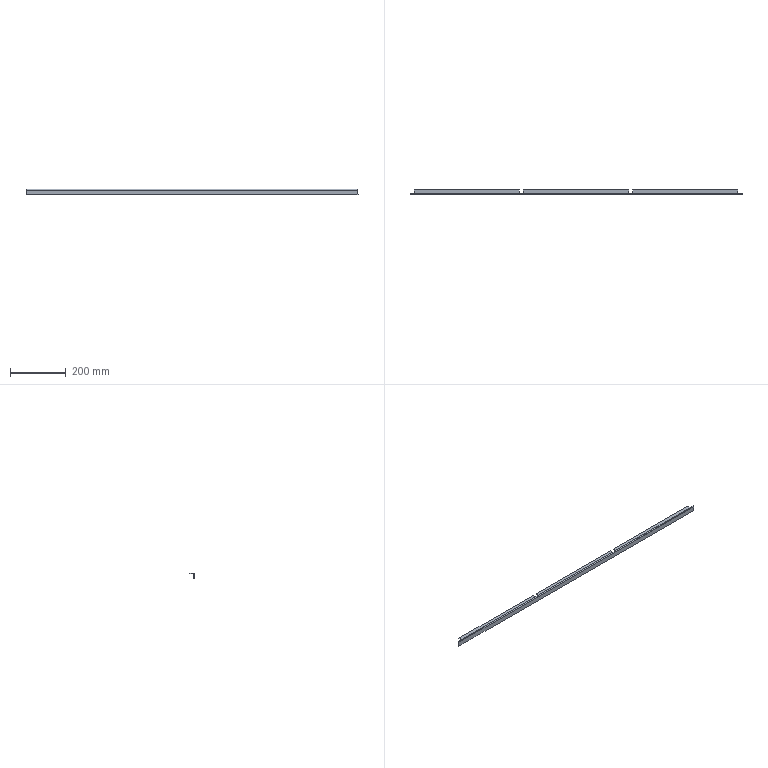Part | SolidWorks | features EdgeFlange 1, FlatPattern 1, ICE 1, LPattern 1, MirrorPattern 1, SMBaseFlange 1, SheetMetal 1 | 1 solid | 28 faces | box 1191 x 15 x 20 mm | volume 92732 mm3 | plane 26 | cylinder 2 | commonest cylinder face diameters 1 x1 6 x1
STEP:
#1=CARTESIAN_POINT('',(-580.5,-4.5,-2.5));
#2=VERTEX_POINT('',#1);
#3=CARTESIAN_POINT('',(-203.5,-4.5,-2.5));
#4=VERTEX_POINT('',#3);
#5=CARTESIAN_POINT('',(-595.5,-4.5,-2.5));
#6=DIRECTION('',(1.,0.,0.));
#7=VECTOR('',#6,1000.);
#8=LINE('',#5,#7);
#9=EDGE_CURVE('',#2,#4,#8,.T.);
#10=ORIENTED_EDGE('',*,*,#9,.F.);
#11=CARTESIAN_POINT('',(-580.5,7.5,-2.5));
#12=VERTEX_POINT('',#11);
#13=CARTESIAN_POINT('',(-580.5,7.5,-2.5));
#14=DIRECTION('',(0.,-1.,0.));
#15=VECTOR('',#14,1000.);
#16=LINE('',#13,#15);
#17=EDGE_CURVE('',#12,#2,#16,.T.);
#18=ORIENTED_EDGE('',*,*,#17,.F.);
#19=CARTESIAN_POINT('',(-203.5,7.5,-2.5));
#20=VERTEX_POINT('',#19);
#21=CARTESIAN_POINT('',(-595.5,7.5,-2.5));
#22=DIRECTION('',(-1.,0.,0.));
#23=VECTOR('',#22,1000.);
#24=LINE('',#21,#23);
#25=EDGE_CURVE('',#20,#12,#24,.T.);
#26=ORIENTED_EDGE('',*,*,#25,.F.);
#27=CARTESIAN_POINT('',(-203.5,7.5,-2.5));
#28=DIRECTION('',(0.,1.,0.));
#29=VECTOR('',#28,1000.);
#30=LINE('',#27,#29);
#31=EDGE_CURVE('',#4,#20,#30,.T.);
#32=ORIENTED_EDGE('',*,*,#31,.F.);
#33=EDGE_LOOP('',(#10,#18,#26,#32));
#34=FACE_OUTER_BOUND('',#33,.T.);
#35=CARTESIAN_POINT('',(595.5,7.5,-2.5));
#36=DIRECTION('',(0.,0.,-1.));
#37=DIRECTION('',(-1.,0.,0.));
#38=AXIS2_PLACEMENT_3D('',#35,#36,#37);
#39=PLANE('',#38);
#40=ADVANCED_FACE('',(#34),#39,.T.);
#41=CARTESIAN_POINT('',(-580.5,7.5,0.));
#42=VERTEX_POINT('',#41);
#43=CARTESIAN_POINT('',(-580.5,-4.5,0.));
#44=VERTEX_POINT('',#43);
#45=CARTESIAN_POINT('',(-580.5,-4.5,0.));
#46=DIRECTION('',(0.,-1.,0.));
#47=VECTOR('',#46,1000.);
#48=LINE('',#45,#47);
#49=EDGE_CURVE('',#42,#44,#48,.T.);
#50=ORIENTED_EDGE('',*,*,#49,.T.);
#51=CARTESIAN_POINT('',(-203.5,-4.5,0.));
#52=VERTEX_POINT('',#51);
#53=CARTESIAN_POINT('',(-595.5,-4.5,0.));
#54=DIRECTION('',(1.,0.,0.));
#55=VECTOR('',#54,1000.);
#56=LINE('',#53,#55);
#57=EDGE_CURVE('',#44,#52,#56,.T.);
#58=ORIENTED_EDGE('',*,*,#57,.T.);
#59=CARTESIAN_POINT('',(-203.5,7.5,0.));
#60=VERTEX_POINT('',#59);
#61=CARTESIAN_POINT('',(-203.5,-4.5,0.));
#62=DIRECTION('',(0.,1.,0.));
#63=VECTOR('',#62,1000.);
#64=LINE('',#61,#63);
#65=EDGE_CURVE('',#52,#60,#64,.T.);
#66=ORIENTED_EDGE('',*,*,#65,.T.);
#67=CARTESIAN_POINT('',(-595.5,7.5,0.));
#68=DIRECTION('',(-1.,0.,0.));
#69=VECTOR('',#68,1000.);
#70=LINE('',#67,#69);
#71=EDGE_CURVE('',#60,#42,#70,.T.);
#72=ORIENTED_EDGE('',*,*,#71,.T.);
#73=EDGE_LOOP('',(#50,#58,#66,#72));
#74=FACE_OUTER_BOUND('',#73,.T.);
#75=CARTESIAN_POINT('',(595.5,7.5,0.));
#76=DIRECTION('',(0.,0.,-1.));
#77=DIRECTION('',(-1.,0.,0.));
#78=AXIS2_PLACEMENT_3D('',#75,#76,#77);
#79=PLANE('',#78);
#80=ADVANCED_FACE('',(#74),#79,.F.);
#81=ORIENTED_EDGE('',*,*,#25,.T.);
#82=CARTESIAN_POINT('',(-580.5,7.5,0.));
#83=DIRECTION('',(0.,0.,-1.));
#84=VECTOR('',#83,1000.);
#85=LINE('',#82,#84);
#86=EDGE_CURVE('',#42,#12,#85,.T.);
#87=ORIENTED_EDGE('',*,*,#86,.F.);
#88=ORIENTED_EDGE('',*,*,#71,.F.);
#89=CARTESIAN_POINT('',(-203.5,7.5,0.));
#90=DIRECTION('',(0.,0.,-1.));
#91=VECTOR('',#90,1000.);
#92=LINE('',#89,#91);
#93=EDGE_CURVE('',#60,#20,#92,.T.);
#94=ORIENTED_EDGE('',*,*,#93,.T.);
#95=EDGE_LOOP('',(#81,#87,#88,#94));
#96=FACE_OUTER_BOUND('',#95,.T.);
#97=CARTESIAN_POINT('',(-595.5,7.5,-2.5));
#98=DIRECTION('',(0.,1.,0.));
#99=DIRECTION('',(0.,0.,1.));
#100=AXIS2_PLACEMENT_3D('',#97,#98,#99);
#101=PLANE('',#100);
#102=ADVANCED_FACE('',(#96),#101,.T.);
#103=CARTESIAN_POINT('',(-188.5,-4.5,-2.5));
#104=VERTEX_POINT('',#103);
#105=CARTESIAN_POINT('',(188.5,-4.5,-2.5));
#106=VERTEX_POINT('',#105);
#107=CARTESIAN_POINT('',(-595.5,-4.5,-2.5));
#108=DIRECTION('',(1.,0.,0.));
#109=VECTOR('',#108,1000.);
#110=LINE('',#107,#109);
#111=EDGE_CURVE('',#104,#106,#110,.T.);
#112=ORIENTED_EDGE('',*,*,#111,.F.);
#113=CARTESIAN_POINT('',(-188.5,7.5,-2.5));
#114=VERTEX_POINT('',#113);
#115=CARTESIAN_POINT('',(-188.5,7.5,-2.5));
#116=DIRECTION('',(0.,-1.,0.));
#117=VECTOR('',#116,1000.);
#118=LINE('',#115,#117);
#119=EDGE_CURVE('',#114,#104,#118,.T.);
#120=ORIENTED_EDGE('',*,*,#119,.F.);
#121=CARTESIAN_POINT('',(188.5,7.5,-2.5));
#122=VERTEX_POINT('',#121);
#123=CARTESIAN_POINT('',(-595.5,7.5,-2.5));
#124=DIRECTION('',(-1.,0.,0.));
#125=VECTOR('',#124,1000.);
#126=LINE('',#123,#125);
#127=EDGE_CURVE('',#122,#114,#126,.T.);
#128=ORIENTED_EDGE('',*,*,#127,.F.);
#129=CARTESIAN_POINT('',(188.5,7.5,-2.5));
#130=DIRECTION('',(0.,-1.,0.));
#131=VECTOR('',#130,1000.);
#132=LINE('',#129,#131);
#133=EDGE_CURVE('',#122,#106,#132,.T.);
#134=ORIENTED_EDGE('',*,*,#133,.T.);
#135=EDGE_LOOP('',(#112,#120,#128,#134));
#136=FACE_OUTER_BOUND('',#135,.T.);
#137=CARTESIAN_POINT('',(595.5,7.5,-2.5));
#138=DIRECTION('',(0.,0.,-1.));
#139=DIRECTION('',(-1.,0.,0.));
#140=AXIS2_PLACEMENT_3D('',#137,#138,#139);
#141=PLANE('',#140);
#142=ADVANCED_FACE('',(#136),#141,.T.);
#143=CARTESIAN_POINT('',(-188.5,7.5,0.));
#144=VERTEX_POINT('',#143);
#145=CARTESIAN_POINT('',(-188.5,-4.5,0.));
#146=VERTEX_POINT('',#145);
#147=CARTESIAN_POINT('',(-188.5,-4.5,0.));
#148=DIRECTION('',(0.,-1.,0.));
#149=VECTOR('',#148,1000.);
#150=LINE('',#147,#149);
#151=EDGE_CURVE('',#144,#146,#150,.T.);
#152=ORIENTED_EDGE('',*,*,#151,.T.);
#153=CARTESIAN_POINT('',(188.5,-4.5,0.));
#154=VERTEX_POINT('',#153);
#155=CARTESIAN_POINT('',(-595.5,-4.5,0.));
#156=DIRECTION('',(1.,0.,0.));
#157=VECTOR('',#156,1000.);
#158=LINE('',#155,#157);
#159=EDGE_CURVE('',#146,#154,#158,.T.);
#160=ORIENTED_EDGE('',*,*,#159,.T.);
#161=CARTESIAN_POINT('',(188.5,7.5,0.));
#162=VERTEX_POINT('',#161);
#163=CARTESIAN_POINT('',(188.5,-4.5,0.));
#164=DIRECTION('',(0.,-1.,0.));
#165=VECTOR('',#164,1000.);
#166=LINE('',#163,#165);
#167=EDGE_CURVE('',#162,#154,#166,.T.);
#168=ORIENTED_EDGE('',*,*,#167,.F.);
#169=CARTESIAN_POINT('',(-595.5,7.5,0.));
#170=DIRECTION('',(-1.,0.,0.));
#171=VECTOR('',#170,1000.);
#172=LINE('',#169,#171);
#173=EDGE_CURVE('',#162,#144,#172,.T.);
#174=ORIENTED_EDGE('',*,*,#173,.T.);
#175=EDGE_LOOP('',(#152,#160,#168,#174));
#176=FACE_OUTER_BOUND('',#175,.T.);
#177=CARTESIAN_POINT('',(595.5,7.5,0.));
#178=DIRECTION('',(0.,0.,-1.));
#179=DIRECTION('',(-1.,0.,0.));
#180=AXIS2_PLACEMENT_3D('',#177,#178,#179);
#181=PLANE('',#180);
#182=ADVANCED_FACE('',(#176),#181,.F.);
#183=ORIENTED_EDGE('',*,*,#127,.T.);
#184=CARTESIAN_POINT('',(-188.5,7.5,0.));
#185=DIRECTION('',(0.,0.,-1.));
#186=VECTOR('',#185,1000.);
#187=LINE('',#184,#186);
#188=EDGE_CURVE('',#144,#114,#187,.T.);
#189=ORIENTED_EDGE('',*,*,#188,.F.);
#190=ORIENTED_EDGE('',*,*,#173,.F.);
#191=CARTESIAN_POINT('',(188.5,7.5,0.));
#192=DIRECTION('',(0.,0.,-1.));
#193=VECTOR('',#192,1000.);
#194=LINE('',#191,#193);
#195=EDGE_CURVE('',#162,#122,#194,.T.);
#196=ORIENTED_EDGE('',*,*,#195,.T.);
#197=EDGE_LOOP('',(#183,#189,#190,#196));
#198=FACE_OUTER_BOUND('',#197,.T.);
#199=CARTESIAN_POINT('',(-595.5,7.5,-2.5));
#200=DIRECTION('',(0.,1.,0.));
#201=DIRECTION('',(0.,0.,1.));
#202=AXIS2_PLACEMENT_3D('',#199,#200,#201);
#203=PLANE('',#202);
#204=ADVANCED_FACE('',(#198),#203,.T.);
#205=CARTESIAN_POINT('',(203.5,-4.5,-2.5));
#206=VERTEX_POINT('',#205);
#207=CARTESIAN_POINT('',(580.5,-4.5,-2.5));
#208=VERTEX_POINT('',#207);
#209=CARTESIAN_POINT('',(-595.5,-4.5,-2.5));
#210=DIRECTION('',(1.,0.,0.));
#211=VECTOR('',#210,1000.);
#212=LINE('',#209,#211);
#213=EDGE_CURVE('',#206,#208,#212,.T.);
#214=ORIENTED_EDGE('',*,*,#213,.F.);
#215=CARTESIAN_POINT('',(203.5,7.5,-2.5));
#216=VERTEX_POINT('',#215);
#217=CARTESIAN_POINT('',(203.5,7.5,-2.5));
#218=DIRECTION('',(0.,1.,0.));
#219=VECTOR('',#218,1000.);
#220=LINE('',#217,#219);
#221=EDGE_CURVE('',#206,#216,#220,.T.);
#222=ORIENTED_EDGE('',*,*,#221,.T.);
#223=CARTESIAN_POINT('',(580.5,7.5,-2.5));
#224=VERTEX_POINT('',#223);
#225=CARTESIAN_POINT('',(-595.5,7.5,-2.5));
#226=DIRECTION('',(-1.,0.,0.));
#227=VECTOR('',#226,1000.);
#228=LINE('',#225,#227);
#229=EDGE_CURVE('',#224,#216,#228,.T.);
#230=ORIENTED_EDGE('',*,*,#229,.F.);
#231=CARTESIAN_POINT('',(580.5,7.5,-2.5));
#232=DIRECTION('',(0.,-1.,0.));
#233=VECTOR('',#232,1000.);
#234=LINE('',#231,#233);
#235=EDGE_CURVE('',#224,#208,#234,.T.);
#236=ORIENTED_EDGE('',*,*,#235,.T.);
#237=EDGE_LOOP('',(#214,#222,#230,#236));
#238=FACE_OUTER_BOUND('',#237,.T.);
#239=CARTESIAN_POINT('',(595.5,7.5,-2.5));
#240=DIRECTION('',(0.,0.,-1.));
#241=DIRECTION('',(-1.,0.,0.));
#242=AXIS2_PLACEMENT_3D('',#239,#240,#241);
#243=PLANE('',#242);
#244=ADVANCED_FACE('',(#238),#243,.T.);
#245=CARTESIAN_POINT('',(203.5,-4.5,0.));
#246=VERTEX_POINT('',#245);
#247=CARTESIAN_POINT('',(203.5,7.5,0.));
#248=VERTEX_POINT('',#247);
#249=CARTESIAN_POINT('',(203.5,-4.5,0.));
#250=DIRECTION('',(0.,1.,0.));
#251=VECTOR('',#250,1000.);
#252=LINE('',#249,#251);
#253=EDGE_CURVE('',#246,#248,#252,.T.);
#254=ORIENTED_EDGE('',*,*,#253,.F.);
#255=CARTESIAN_POINT('',(580.5,-4.5,0.));
#256=VERTEX_POINT('',#255);
#257=CARTESIAN_POINT('',(-595.5,-4.5,0.));
#258=DIRECTION('',(1.,0.,0.));
#259=VECTOR('',#258,1000.);
#260=LINE('',#257,#259);
#261=EDGE_CURVE('',#246,#256,#260,.T.);
#262=ORIENTED_EDGE('',*,*,#261,.T.);
#263=CARTESIAN_POINT('',(580.5,7.5,0.));
#264=VERTEX_POINT('',#263);
#265=CARTESIAN_POINT('',(580.5,-4.5,0.));
#266=DIRECTION('',(0.,-1.,0.));
#267=VECTOR('',#266,1000.);
#268=LINE('',#265,#267);
#269=EDGE_CURVE('',#264,#256,#268,.T.);
#270=ORIENTED_EDGE('',*,*,#269,.F.);
#271=CARTESIAN_POINT('',(-595.5,7.5,0.));
#272=DIRECTION('',(-1.,0.,0.));
#273=VECTOR('',#272,1000.);
#274=LINE('',#271,#273);
#275=EDGE_CURVE('',#264,#248,#274,.T.);
#276=ORIENTED_EDGE('',*,*,#275,.T.);
#277=EDGE_LOOP('',(#254,#262,#270,#276));
#278=FACE_OUTER_BOUND('',#277,.T.);
#279=CARTESIAN_POINT('',(595.5,7.5,0.));
#280=DIRECTION('',(0.,0.,-1.));
#281=DIRECTION('',(-1.,0.,0.));
#282=AXIS2_PLACEMENT_3D('',#279,#280,#281);
#283=PLANE('',#282);
#284=ADVANCED_FACE('',(#278),#283,.F.);
#285=ORIENTED_EDGE('',*,*,#229,.T.);
#286=CARTESIAN_POINT('',(203.5,7.5,0.));
#287=DIRECTION('',(0.,0.,-1.));
#288=VECTOR('',#287,1000.);
#289=LINE('',#286,#288);
#290=EDGE_CURVE('',#248,#216,#289,.T.);
#291=ORIENTED_EDGE('',*,*,#290,.F.);
#292=ORIENTED_EDGE('',*,*,#275,.F.);
#293=CARTESIAN_POINT('',(580.5,7.5,0.));
#294=DIRECTION('',(0.,0.,-1.));
#295=VECTOR('',#294,1000.);
#296=LINE('',#293,#295);
#297=EDGE_CURVE('',#264,#224,#296,.T.);
#298=ORIENTED_EDGE('',*,*,#297,.T.);
#299=EDGE_LOOP('',(#285,#291,#292,#298));
#300=FACE_OUTER_BOUND('',#299,.T.);
#301=CARTESIAN_POINT('',(-595.5,7.5,-2.5));
#302=DIRECTION('',(0.,1.,0.));
#303=DIRECTION('',(0.,0.,1.));
#304=AXIS2_PLACEMENT_3D('',#301,#302,#303);
#305=PLANE('',#304);
#306=ADVANCED_FACE('',(#300),#305,.T.);
#307=CARTESIAN_POINT('',(595.5,-5.,-3.));
#308=VERTEX_POINT('',#307);
#309=CARTESIAN_POINT('',(595.5,-7.5,-3.));
#310=VERTEX_POINT('',#309);
#311=CARTESIAN_POINT('',(595.5,-7.5,-3.));
#312=DIRECTION('',(0.,-1.,0.));
#313=VECTOR('',#312,1000.);
#314=LINE('',#311,#313);
#315=EDGE_CURVE('',#308,#310,#314,.T.);
#316=ORIENTED_EDGE('',*,*,#315,.F.);
#317=CARTESIAN_POINT('',(595.5,-4.5,-2.5));
#318=VERTEX_POINT('',#317);
#319=CARTESIAN_POINT('',(595.5,-4.5,-3.));
#320=DIRECTION('',(1.,0.,0.));
#321=DIRECTION('',(0.,0.,1.));
#322=AXIS2_PLACEMENT_3D('',#319,#320,#321);
#323=CIRCLE('',#322,0.5);
#324=EDGE_CURVE('',#318,#308,#323,.T.);
#325=ORIENTED_EDGE('',*,*,#324,.F.);
#326=CARTESIAN_POINT('',(595.5,-4.5,0.));
#327=VERTEX_POINT('',#326);
#328=CARTESIAN_POINT('',(595.5,-4.5,-2.5));
#329=DIRECTION('',(0.,0.,1.));
#330=VECTOR('',#329,1000.);
#331=LINE('',#328,#330);
#332=EDGE_CURVE('',#318,#327,#331,.T.);
#333=ORIENTED_EDGE('',*,*,#332,.T.);
#334=CARTESIAN_POINT('',(595.5,-4.5,-3.));
#335=DIRECTION('',(1.,0.,0.));
#336=DIRECTION('',(0.,0.,1.));
#337=AXIS2_PLACEMENT_3D('',#334,#335,#336);
#338=CIRCLE('',#337,3.);
#339=EDGE_CURVE('',#327,#310,#338,.T.);
#340=ORIENTED_EDGE('',*,*,#339,.T.);
#341=EDGE_LOOP('',(#316,#325,#333,#340));
#342=FACE_OUTER_BOUND('',#341,.T.);
#343=CARTESIAN_POINT('',(595.5,-4.5,-3.));
#344=DIRECTION('',(1.,0.,0.));
#345=DIRECTION('',(0.,0.,-1.));
#346=AXIS2_PLACEMENT_3D('',#343,#344,#345);
#347=PLANE('',#346);
#348=ADVANCED_FACE('',(#342),#347,.T.);
#349=CARTESIAN_POINT('',(-595.5,-4.5,0.));
#350=VERTEX_POINT('',#349);
#351=CARTESIAN_POINT('',(-595.5,-4.5,0.));
#352=DIRECTION('',(1.,0.,0.));
#353=VECTOR('',#352,1000.);
#354=LINE('',#351,#353);
#355=EDGE_CURVE('',#350,#44,#354,.T.);
#356=ORIENTED_EDGE('',*,*,#355,.F.);
#357=CARTESIAN_POINT('',(-595.5,-7.5,-3.));
#358=VERTEX_POINT('',#357);
#359=CARTESIAN_POINT('',(-595.5,-4.5,-3.));
#360=DIRECTION('',(-1.,0.,0.));
#361=DIRECTION('',(0.,0.,1.));
#362=AXIS2_PLACEMENT_3D('',#359,#360,#361);
#363=CIRCLE('',#362,3.);
#364=EDGE_CURVE('',#358,#350,#363,.T.);
#365=ORIENTED_EDGE('',*,*,#364,.F.);
#366=CARTESIAN_POINT('',(-595.5,-7.5,-3.));
#367=DIRECTION('',(-1.,0.,0.));
#368=VECTOR('',#367,1000.);
#369=LINE('',#366,#368);
#370=EDGE_CURVE('',#310,#358,#369,.T.);
#371=ORIENTED_EDGE('',*,*,#370,.F.);
#372=ORIENTED_EDGE('',*,*,#339,.F.);
#373=CARTESIAN_POINT('',(595.5,-4.5,0.));
#374=DIRECTION('',(1.,0.,0.));
#375=VECTOR('',#374,1000.);
#376=LINE('',#373,#375);
#377=EDGE_CURVE('',#256,#327,#376,.T.);
#378=ORIENTED_EDGE('',*,*,#377,.F.);
#379=ORIENTED_EDGE('',*,*,#261,.F.);
#380=CARTESIAN_POINT('',(203.5,-4.5,0.));
#381=DIRECTION('',(1.,0.,0.));
#382=VECTOR('',#381,1000.);
#383=LINE('',#380,#382);
#384=EDGE_CURVE('',#154,#246,#383,.T.);
#385=ORIENTED_EDGE('',*,*,#384,.F.);
#386=ORIENTED_EDGE('',*,*,#159,.F.);
#387=CARTESIAN_POINT('',(-203.5,-4.5,0.));
#388=DIRECTION('',(-1.,0.,0.));
#389=VECTOR('',#388,1000.);
#390=LINE('',#387,#389);
#391=EDGE_CURVE('',#146,#52,#390,.T.);
#392=ORIENTED_EDGE('',*,*,#391,.T.);
#393=ORIENTED_EDGE('',*,*,#57,.F.);
#394=EDGE_LOOP('',(#356,#365,#371,#372,#378,#379,#385,#386,#392,#393));
#395=FACE_OUTER_BOUND('',#394,.T.);
#396=CARTESIAN_POINT('',(-595.5,-4.5,-3.));
#397=DIRECTION('',(-1.,0.,0.));
#398=DIRECTION('',(0.,-1.,0.));
#399=AXIS2_PLACEMENT_3D('',#396,#397,#398);
#400=CYLINDRICAL_SURFACE('',#399,3.);
#401=ADVANCED_FACE('',(#395),#400,.T.);
#402=CARTESIAN_POINT('',(-595.5,-5.,-3.));
#403=VERTEX_POINT('',#402);
#404=CARTESIAN_POINT('',(-595.5,-4.5,-2.5));
#405=VERTEX_POINT('',#404);
#406=CARTESIAN_POINT('',(-595.5,-4.5,-3.));
#407=DIRECTION('',(-1.,0.,0.));
#408=DIRECTION('',(0.,0.,1.));
#409=AXIS2_PLACEMENT_3D('',#406,#407,#408);
#410=CIRCLE('',#409,0.5);
#411=EDGE_CURVE('',#403,#405,#410,.T.);
#412=ORIENTED_EDGE('',*,*,#411,.F.);
#413=CARTESIAN_POINT('',(-595.5,-5.,-3.));
#414=DIRECTION('',(0.,-1.,0.));
#415=VECTOR('',#414,1000.);
#416=LINE('',#413,#415);
#417=EDGE_CURVE('',#403,#358,#416,.T.);
#418=ORIENTED_EDGE('',*,*,#417,.T.);
#419=ORIENTED_EDGE('',*,*,#364,.T.);
#420=CARTESIAN_POINT('',(-595.5,-4.5,-2.5));
#421=DIRECTION('',(0.,0.,1.));
#422=VECTOR('',#421,1000.);
#423=LINE('',#420,#422);
#424=EDGE_CURVE('',#405,#350,#423,.T.);
#425=ORIENTED_EDGE('',*,*,#424,.F.);
#426=EDGE_LOOP('',(#412,#418,#419,#425));
#427=FACE_OUTER_BOUND('',#426,.T.);
#428=CARTESIAN_POINT('',(-595.5,-4.5,-3.));
#429=DIRECTION('',(1.,0.,0.));
#430=DIRECTION('',(0.,0.,-1.));
#431=AXIS2_PLACEMENT_3D('',#428,#429,#430);
#432=PLANE('',#431);
#433=ADVANCED_FACE('',(#427),#432,.F.);
#434=CARTESIAN_POINT('',(-595.5,-4.5,-2.5));
#435=DIRECTION('',(1.,0.,0.));
#436=VECTOR('',#435,1000.);
#437=LINE('',#434,#436);
#438=EDGE_CURVE('',#405,#2,#437,.T.);
#439=ORIENTED_EDGE('',*,*,#438,.T.);
#440=ORIENTED_EDGE('',*,*,#9,.T.);
#441=CARTESIAN_POINT('',(595.5,-4.5,-2.5));
#442=DIRECTION('',(-1.,0.,0.));
#443=VECTOR('',#442,1000.);
#444=LINE('',#441,#443);
#445=EDGE_CURVE('',#104,#4,#444,.T.);
#446=ORIENTED_EDGE('',*,*,#445,.F.);
#447=ORIENTED_EDGE('',*,*,#111,.T.);
#448=CARTESIAN_POINT('',(595.5,-4.5,-2.5));
#449=DIRECTION('',(1.,0.,0.));
#450=VECTOR('',#449,1000.);
#451=LINE('',#448,#450);
#452=EDGE_CURVE('',#106,#206,#451,.T.);
#453=ORIENTED_EDGE('',*,*,#452,.T.);
#454=ORIENTED_EDGE('',*,*,#213,.T.);
#455=CARTESIAN_POINT('',(595.5,-4.5,-2.5));
#456=DIRECTION('',(1.,0.,0.));
#457=VECTOR('',#456,1000.);
#458=LINE('',#455,#457);
#459=EDGE_CURVE('',#208,#318,#458,.T.);
#460=ORIENTED_EDGE('',*,*,#459,.T.);
#461=ORIENTED_EDGE('',*,*,#324,.T.);
#462=CARTESIAN_POINT('',(595.5,-5.,-3.));
#463=DIRECTION('',(-1.,0.,0.));
#464=VECTOR('',#463,1000.);
#465=LINE('',#462,#464);
#466=EDGE_CURVE('',#308,#403,#465,.T.);
#467=ORIENTED_EDGE('',*,*,#466,.T.);
#468=ORIENTED_EDGE('',*,*,#411,.T.);
#469=EDGE_LOOP('',(#439,#440,#446,#447,#453,#454,#460,#461,#467,#468));
#470=FACE_OUTER_BOUND('',#469,.T.);
#471=CARTESIAN_POINT('',(-595.5,-4.5,-3.));
#472=DIRECTION('',(-1.,0.,0.));
#473=DIRECTION('',(0.,-1.,0.));
#474=AXIS2_PLACEMENT_3D('',#471,#472,#473);
#475=CYLINDRICAL_SURFACE('',#474,0.5);
#476=ADVANCED_FACE('',(#470),#475,.F.);
#477=CARTESIAN_POINT('',(-595.5,-7.5,-20.));
#478=VERTEX_POINT('',#477);
#479=CARTESIAN_POINT('',(-595.5,-7.5,-2.5));
#480=DIRECTION('',(0.,0.,1.));
#481=VECTOR('',#480,1000.);
#482=LINE('',#479,#481);
#483=EDGE_CURVE('',#478,#358,#482,.T.);
#484=ORIENTED_EDGE('',*,*,#483,.T.);
#485=ORIENTED_EDGE('',*,*,#417,.F.);
#486=CARTESIAN_POINT('',(-595.5,-5.,-20.));
#487=VERTEX_POINT('',#486);
#488=CARTESIAN_POINT('',(-595.5,-5.,-2.5));
#489=DIRECTION('',(0.,0.,1.));
#490=VECTOR('',#489,1000.);
#491=LINE('',#488,#490);
#492=EDGE_CURVE('',#487,#403,#491,.T.);
#493=ORIENTED_EDGE('',*,*,#492,.F.);
#494=CARTESIAN_POINT('',(-595.5,-7.5,-20.));
#495=DIRECTION('',(0.,1.,0.));
#496=VECTOR('',#495,1000.);
#497=LINE('',#494,#496);
#498=EDGE_CURVE('',#478,#487,#497,.T.);
#499=ORIENTED_EDGE('',*,*,#498,.F.);
#500=EDGE_LOOP('',(#484,#485,#493,#499));
#501=FACE_OUTER_BOUND('',#500,.T.);
#502=CARTESIAN_POINT('',(-595.5,-7.5,-2.5));
#503=DIRECTION('',(-1.,0.,0.));
#504=DIRECTION('',(0.,0.,1.));
#505=AXIS2_PLACEMENT_3D('',#502,#503,#504);
#506=PLANE('',#505);
#507=ADVANCED_FACE('',(#501),#506,.T.);
#508=CARTESIAN_POINT('',(595.5,-5.,-20.));
#509=VERTEX_POINT('',#508);
#510=CARTESIAN_POINT('',(595.5,-5.,-2.5));
#511=DIRECTION('',(0.,0.,-1.));
#512=VECTOR('',#511,1000.);
#513=LINE('',#510,#512);
#514=EDGE_CURVE('',#308,#509,#513,.T.);
#515=ORIENTED_EDGE('',*,*,#514,.F.);
#516=ORIENTED_EDGE('',*,*,#315,.T.);
#517=CARTESIAN_POINT('',(595.5,-7.5,-20.));
#518=VERTEX_POINT('',#517);
#519=CARTESIAN_POINT('',(595.5,-7.5,-20.));
#520=DIRECTION('',(0.,0.,-1.));
#521=VECTOR('',#520,1000.);
#522=LINE('',#519,#521);
#523=EDGE_CURVE('',#310,#518,#522,.T.);
#524=ORIENTED_EDGE('',*,*,#523,.T.);
#525=CARTESIAN_POINT('',(595.5,-7.5,-20.));
#526=DIRECTION('',(0.,1.,0.));
#527=VECTOR('',#526,1000.);
#528=LINE('',#525,#527);
#529=EDGE_CURVE('',#518,#509,#528,.T.);
#530=ORIENTED_EDGE('',*,*,#529,.T.);
#531=EDGE_LOOP('',(#515,#516,#524,#530));
#532=FACE_OUTER_BOUND('',#531,.T.);
#533=CARTESIAN_POINT('',(595.5,-7.5,-20.));
#534=DIRECTION('',(1.,0.,0.));
#535=DIRECTION('',(0.,0.,-1.));
#536=AXIS2_PLACEMENT_3D('',#533,#534,#535);
#537=PLANE('',#536);
#538=ADVANCED_FACE('',(#532),#537,.T.);
#539=ORIENTED_EDGE('',*,*,#523,.F.);
#540=ORIENTED_EDGE('',*,*,#370,.T.);
#541=ORIENTED_EDGE('',*,*,#483,.F.);
#542=CARTESIAN_POINT('',(-595.5,-7.5,-20.));
#543=DIRECTION('',(-1.,0.,0.));
#544=VECTOR('',#543,1000.);
#545=LINE('',#542,#544);
#546=EDGE_CURVE('',#518,#478,#545,.T.);
#547=ORIENTED_EDGE('',*,*,#546,.F.);
#548=EDGE_LOOP('',(#539,#540,#541,#547));
#549=FACE_OUTER_BOUND('',#548,.T.);
#550=CARTESIAN_POINT('',(-595.5,-7.5,-2.5));
#551=DIRECTION('',(0.,-1.,0.));
#552=DIRECTION('',(0.,0.,-1.));
#553=AXIS2_PLACEMENT_3D('',#550,#551,#552);
#554=PLANE('',#553);
#555=ADVANCED_FACE('',(#549),#554,.T.);
#556=ORIENTED_EDGE('',*,*,#466,.F.);
#557=ORIENTED_EDGE('',*,*,#514,.T.);
#558=CARTESIAN_POINT('',(-595.5,-5.,-20.));
#559=DIRECTION('',(-1.,0.,0.));
#560=VECTOR('',#559,1000.);
#561=LINE('',#558,#560);
#562=EDGE_CURVE('',#509,#487,#561,.T.);
#563=ORIENTED_EDGE('',*,*,#562,.T.);
#564=ORIENTED_EDGE('',*,*,#492,.T.);
#565=EDGE_LOOP('',(#556,#557,#563,#564));
#566=FACE_OUTER_BOUND('',#565,.T.);
#567=CARTESIAN_POINT('',(-595.5,-5.,-2.5));
#568=DIRECTION('',(0.,-1.,0.));
#569=DIRECTION('',(0.,0.,-1.));
#570=AXIS2_PLACEMENT_3D('',#567,#568,#569);
#571=PLANE('',#570);
#572=ADVANCED_FACE('',(#566),#571,.F.);
#573=ORIENTED_EDGE('',*,*,#562,.F.);
#574=ORIENTED_EDGE('',*,*,#529,.F.);
#575=ORIENTED_EDGE('',*,*,#546,.T.);
#576=ORIENTED_EDGE('',*,*,#498,.T.);
#577=EDGE_LOOP('',(#573,#574,#575,#576));
#578=FACE_OUTER_BOUND('',#577,.T.);
#579=CARTESIAN_POINT('',(-595.5,-7.5,-20.));
#580=DIRECTION('',(0.,0.,-1.));
#581=DIRECTION('',(0.,1.,0.));
#582=AXIS2_PLACEMENT_3D('',#579,#580,#581);
#583=PLANE('',#582);
#584=ADVANCED_FACE('',(#578),#583,.T.);
#585=ORIENTED_EDGE('',*,*,#297,.F.);
#586=ORIENTED_EDGE('',*,*,#269,.T.);
#587=CARTESIAN_POINT('',(580.5,-4.5,0.));
#588=DIRECTION('',(0.,0.,-1.));
#589=VECTOR('',#588,1000.);
#590=LINE('',#587,#589);
#591=EDGE_CURVE('',#256,#208,#590,.T.);
#592=ORIENTED_EDGE('',*,*,#591,.T.);
#593=ORIENTED_EDGE('',*,*,#235,.F.);
#594=EDGE_LOOP('',(#585,#586,#592,#593));
#595=FACE_OUTER_BOUND('',#594,.T.);
#596=CARTESIAN_POINT('',(580.5,-4.5,0.));
#597=DIRECTION('',(1.,0.,0.));
#598=DIRECTION('',(0.,-1.,0.));
#599=AXIS2_PLACEMENT_3D('',#596,#597,#598);
#600=PLANE('',#599);
#601=ADVANCED_FACE('',(#595),#600,.T.);
#602=ORIENTED_EDGE('',*,*,#377,.T.);
#603=ORIENTED_EDGE('',*,*,#332,.F.);
#604=ORIENTED_EDGE('',*,*,#459,.F.);
#605=ORIENTED_EDGE('',*,*,#591,.F.);
#606=EDGE_LOOP('',(#602,#603,#604,#605));
#607=FACE_OUTER_BOUND('',#606,.T.);
#608=CARTESIAN_POINT('',(595.5,-4.5,0.));
#609=DIRECTION('',(0.,1.,0.));
#610=DIRECTION('',(1.,0.,0.));
#611=AXIS2_PLACEMENT_3D('',#608,#609,#610);
#612=PLANE('',#611);
#613=ADVANCED_FACE('',(#607),#612,.T.);
#614=ORIENTED_EDGE('',*,*,#195,.F.);
#615=ORIENTED_EDGE('',*,*,#167,.T.);
#616=CARTESIAN_POINT('',(188.5,-4.5,0.));
#617=DIRECTION('',(0.,0.,-1.));
#618=VECTOR('',#617,1000.);
#619=LINE('',#616,#618);
#620=EDGE_CURVE('',#154,#106,#619,.T.);
#621=ORIENTED_EDGE('',*,*,#620,.T.);
#622=ORIENTED_EDGE('',*,*,#133,.F.);
#623=EDGE_LOOP('',(#614,#615,#621,#622));
#624=FACE_OUTER_BOUND('',#623,.T.);
#625=CARTESIAN_POINT('',(188.5,-4.5,0.));
#626=DIRECTION('',(1.,0.,0.));
#627=DIRECTION('',(0.,-1.,0.));
#628=AXIS2_PLACEMENT_3D('',#625,#626,#627);
#629=PLANE('',#628);
#630=ADVANCED_FACE('',(#624),#629,.T.);
#631=ORIENTED_EDGE('',*,*,#620,.F.);
#632=ORIENTED_EDGE('',*,*,#384,.T.);
#633=CARTESIAN_POINT('',(203.5,-4.5,0.));
#634=DIRECTION('',(0.,0.,-1.));
#635=VECTOR('',#634,1000.);
#636=LINE('',#633,#635);
#637=EDGE_CURVE('',#246,#206,#636,.T.);
#638=ORIENTED_EDGE('',*,*,#637,.T.);
#639=ORIENTED_EDGE('',*,*,#452,.F.);
#640=EDGE_LOOP('',(#631,#632,#638,#639));
#641=FACE_OUTER_BOUND('',#640,.T.);
#642=CARTESIAN_POINT('',(203.5,-4.5,0.));
#643=DIRECTION('',(0.,1.,0.));
#644=DIRECTION('',(1.,0.,0.));
#645=AXIS2_PLACEMENT_3D('',#642,#643,#644);
#646=PLANE('',#645);
#647=ADVANCED_FACE('',(#641),#646,.T.);
#648=ORIENTED_EDGE('',*,*,#637,.F.);
#649=ORIENTED_EDGE('',*,*,#253,.T.);
#650=ORIENTED_EDGE('',*,*,#290,.T.);
#651=ORIENTED_EDGE('',*,*,#221,.F.);
#652=EDGE_LOOP('',(#648,#649,#650,#651));
#653=FACE_OUTER_BOUND('',#652,.T.);
#654=CARTESIAN_POINT('',(203.5,-4.5,0.));
#655=DIRECTION('',(-1.,0.,0.));
#656=DIRECTION('',(0.,1.,0.));
#657=AXIS2_PLACEMENT_3D('',#654,#655,#656);
#658=PLANE('',#657);
#659=ADVANCED_FACE('',(#653),#658,.T.);
#660=CARTESIAN_POINT('',(-203.5,-4.5,0.));
#661=DIRECTION('',(0.,0.,-1.));
#662=VECTOR('',#661,1000.);
#663=LINE('',#660,#662);
#664=EDGE_CURVE('',#52,#4,#663,.T.);
#665=ORIENTED_EDGE('',*,*,#664,.F.);
#666=ORIENTED_EDGE('',*,*,#391,.F.);
#667=CARTESIAN_POINT('',(-188.5,-4.5,0.));
#668=DIRECTION('',(0.,0.,-1.));
#669=VECTOR('',#668,1000.);
#670=LINE('',#667,#669);
#671=EDGE_CURVE('',#146,#104,#670,.T.);
#672=ORIENTED_EDGE('',*,*,#671,.T.);
#673=ORIENTED_EDGE('',*,*,#445,.T.);
#674=EDGE_LOOP('',(#665,#666,#672,#673));
#675=FACE_OUTER_BOUND('',#674,.T.);
#676=CARTESIAN_POINT('',(-203.5,-4.5,0.));
#677=DIRECTION('',(0.,-1.,0.));
#678=DIRECTION('',(-1.,0.,0.));
#679=AXIS2_PLACEMENT_3D('',#676,#677,#678);
#680=PLANE('',#679);
#681=ADVANCED_FACE('',(#675),#680,.F.);
#682=ORIENTED_EDGE('',*,*,#671,.F.);
#683=ORIENTED_EDGE('',*,*,#151,.F.);
#684=ORIENTED_EDGE('',*,*,#188,.T.);
#685=ORIENTED_EDGE('',*,*,#119,.T.);
#686=EDGE_LOOP('',(#682,#683,#684,#685));
#687=FACE_OUTER_BOUND('',#686,.T.);
#688=CARTESIAN_POINT('',(-188.5,-4.5,0.));
#689=DIRECTION('',(1.,0.,0.));
#690=DIRECTION('',(0.,-1.,0.));
#691=AXIS2_PLACEMENT_3D('',#688,#689,#690);
#692=PLANE('',#691);
#693=ADVANCED_FACE('',(#687),#692,.F.);
#694=ORIENTED_EDGE('',*,*,#65,.F.);
#695=ORIENTED_EDGE('',*,*,#664,.T.);
#696=ORIENTED_EDGE('',*,*,#31,.T.);
#697=ORIENTED_EDGE('',*,*,#93,.F.);
#698=EDGE_LOOP('',(#694,#695,#696,#697));
#699=FACE_OUTER_BOUND('',#698,.T.);
#700=CARTESIAN_POINT('',(-203.5,-4.5,0.));
#701=DIRECTION('',(-1.,0.,0.));
#702=DIRECTION('',(0.,1.,0.));
#703=AXIS2_PLACEMENT_3D('',#700,#701,#702);
#704=PLANE('',#703);
#705=ADVANCED_FACE('',(#699),#704,.F.);
#706=ORIENTED_EDGE('',*,*,#424,.T.);
#707=ORIENTED_EDGE('',*,*,#355,.T.);
#708=CARTESIAN_POINT('',(-580.5,-4.5,0.));
#709=DIRECTION('',(0.,0.,-1.));
#710=VECTOR('',#709,1000.);
#711=LINE('',#708,#710);
#712=EDGE_CURVE('',#44,#2,#711,.T.);
#713=ORIENTED_EDGE('',*,*,#712,.T.);
#714=ORIENTED_EDGE('',*,*,#438,.F.);
#715=EDGE_LOOP('',(#706,#707,#713,#714));
#716=FACE_OUTER_BOUND('',#715,.T.);
#717=CARTESIAN_POINT('',(-595.5,-4.5,0.));
#718=DIRECTION('',(0.,-1.,0.));
#719=DIRECTION('',(-1.,0.,0.));
#720=AXIS2_PLACEMENT_3D('',#717,#718,#719);
#721=PLANE('',#720);
#722=ADVANCED_FACE('',(#716),#721,.F.);
#723=ORIENTED_EDGE('',*,*,#49,.F.);
#724=ORIENTED_EDGE('',*,*,#86,.T.);
#725=ORIENTED_EDGE('',*,*,#17,.T.);
#726=ORIENTED_EDGE('',*,*,#712,.F.);
#727=EDGE_LOOP('',(#723,#724,#725,#726));
#728=FACE_OUTER_BOUND('',#727,.T.);
#729=CARTESIAN_POINT('',(-580.5,-4.5,0.));
#730=DIRECTION('',(1.,0.,0.));
#731=DIRECTION('',(0.,-1.,0.));
#732=AXIS2_PLACEMENT_3D('',#729,#730,#731);
#733=PLANE('',#732);
#734=ADVANCED_FACE('',(#728),#733,.F.);
#735=CLOSED_SHELL('',(#40,#80,#102,#142,#182,#204,#244,#284,#306,#348,#401,#433,#476,#507,#538,#555,#572,#584,#601,#613,#630,#647,#659,#681,#693,#705,#722,#734));
#736=MANIFOLD_SOLID_BREP('',#735);
#737=CARTESIAN_POINT('',(0.,0.,0.));
#738=DIRECTION('',(0.,0.,1.));
#739=DIRECTION('',(1.,0.,0.));
#740=AXIS2_PLACEMENT_3D('',#737,#738,#739);
#741=(LENGTH_UNIT()NAMED_UNIT(*)SI_UNIT(.MILLI.,.METRE.));
#742=UNCERTAINTY_MEASURE_WITH_UNIT(LENGTH_MEASURE(0.00001),#741,'','');
#743=(NAMED_UNIT(*)PLANE_ANGLE_UNIT()SI_UNIT($,.RADIAN.));
#744=(NAMED_UNIT(*)SI_UNIT($,.STERADIAN.)SOLID_ANGLE_UNIT());
#745=(GEOMETRIC_REPRESENTATION_CONTEXT(3)GLOBAL_UNCERTAINTY_ASSIGNED_CONTEXT((#742))GLOBAL_UNIT_ASSIGNED_CONTEXT((#741,#743,#744))REPRESENTATION_CONTEXT('',''));
#746=ADVANCED_BREP_SHAPE_REPRESENTATION('',(#736,#740),#745);